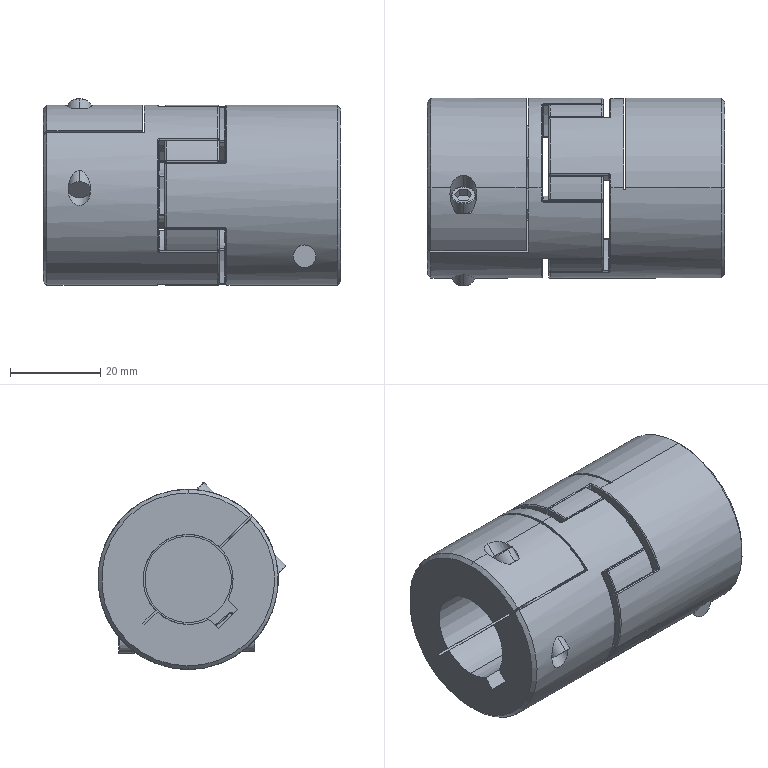Part | SolidWorks | features BaseBody 3 | 3 solids | 414 faces | box 66 x 41.729 x 41.508 mm | volume 63397 mm3 | torus 145 | cylinder 137 | sphere 58 | plane 57 | spline 12 | cone 5 | commonest cylinder face diameters 0.48 x58 24 x36 40 x13 5 x10 20 x5 14 x4